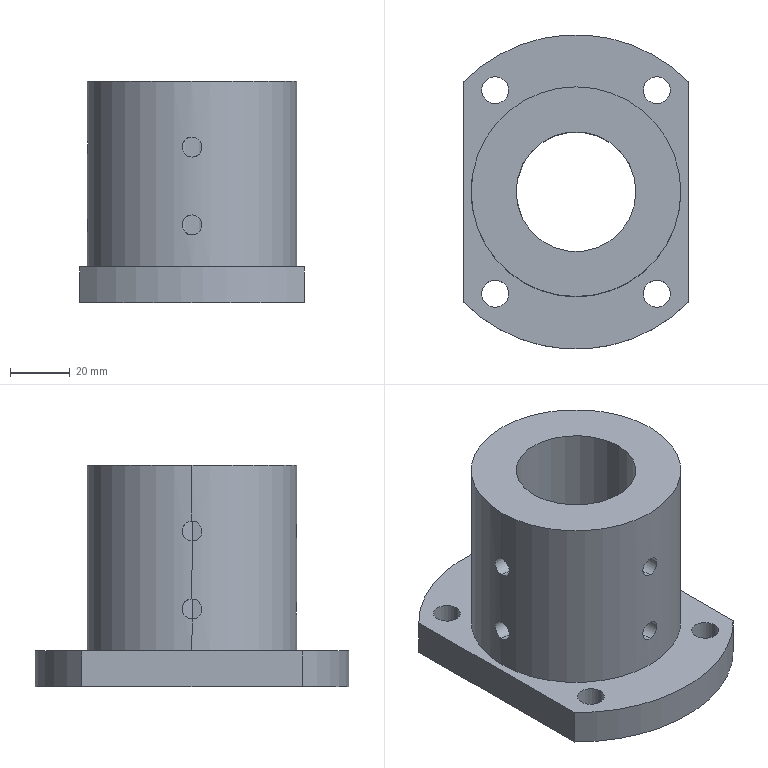Part | NX | features BREP 1 | 1 solid | 27 faces | box 75 x 105 x 74 mm | volume 226168 mm3 | cylinder 22 | plane 5 | commonest cylinder face diameters 6.647 x8 9 x8 40 x2 70 x2 105 x2
STEP:
#1=CARTESIAN_POINT('',(35.,0.,0.));
#2=VERTEX_POINT('',#1);
#3=CARTESIAN_POINT('',(-35.,0.,0.));
#4=VERTEX_POINT('',#3);
#5=CARTESIAN_POINT('',(0.,0.,0.));
#6=DIRECTION('',(0.,0.,1.));
#7=DIRECTION('',(1.,0.,0.));
#8=AXIS2_PLACEMENT_3D('',#5,#6,#7);
#9=CIRCLE('',#8,35.);
#10=EDGE_CURVE('',#2,#4,#9,.T.);
#11=ORIENTED_EDGE('',*,*,#10,.T.);
#12=CARTESIAN_POINT('',(-35.,0.,10.677));
#13=VERTEX_POINT('',#12);
#14=CARTESIAN_POINT('',(-35.,0.,0.));
#15=DIRECTION('',(0.,0.,1.));
#16=VECTOR('',#15,1000.);
#17=LINE('',#14,#16);
#18=EDGE_CURVE('',#4,#13,#17,.T.);
#19=ORIENTED_EDGE('',*,*,#18,.T.);
#20=CARTESIAN_POINT('',(-35.,0.,17.323));
#21=VERTEX_POINT('',#20);
#22=CARTESIAN_POINT('',(-35.,0.,10.677));
#23=CARTESIAN_POINT('',(-35.,0.874,10.677));
#24=CARTESIAN_POINT('',(-34.921,2.604,11.398));
#25=CARTESIAN_POINT('',(-34.802,3.684,14.));
#26=CARTESIAN_POINT('',(-34.921,2.603,16.603));
#27=CARTESIAN_POINT('',(-35.,0.8744,17.323));
#28=CARTESIAN_POINT('',(-35.,0.,17.323));
#29=B_SPLINE_CURVE_WITH_KNOTS('',3,(#22,#23,#24,#25,#26,#27,#28),.UNSPECIFIED.,.F.,.F.,(4,1,1,1,4),(0.,0.25,0.5,0.75,1.),.UNSPECIFIED.);
#30=EDGE_CURVE('',#13,#21,#29,.T.);
#31=ORIENTED_EDGE('',*,*,#30,.T.);
#32=CARTESIAN_POINT('',(-35.,0.,36.676));
#33=VERTEX_POINT('',#32);
#34=CARTESIAN_POINT('',(-35.,0.,0.));
#35=DIRECTION('',(0.,0.,1.));
#36=VECTOR('',#35,1000.);
#37=LINE('',#34,#36);
#38=EDGE_CURVE('',#21,#33,#37,.T.);
#39=ORIENTED_EDGE('',*,*,#38,.T.);
#40=CARTESIAN_POINT('',(-35.,0.,43.324));
#41=VERTEX_POINT('',#40);
#42=CARTESIAN_POINT('',(-35.,0.,36.676));
#43=CARTESIAN_POINT('',(-35.,0.874,36.676));
#44=CARTESIAN_POINT('',(-34.921,2.604,37.398));
#45=CARTESIAN_POINT('',(-34.802,3.684,40.));
#46=CARTESIAN_POINT('',(-34.921,2.603,42.603));
#47=CARTESIAN_POINT('',(-35.,0.8744,43.324));
#48=CARTESIAN_POINT('',(-35.,0.,43.324));
#49=B_SPLINE_CURVE_WITH_KNOTS('',3,(#42,#43,#44,#45,#46,#47,#48),.UNSPECIFIED.,.F.,.F.,(4,1,1,1,4),(0.,0.25,0.5,0.75,1.),.UNSPECIFIED.);
#50=EDGE_CURVE('',#33,#41,#49,.T.);
#51=ORIENTED_EDGE('',*,*,#50,.T.);
#52=CARTESIAN_POINT('',(-35.,0.,62.));
#53=VERTEX_POINT('',#52);
#54=CARTESIAN_POINT('',(-35.,0.,0.));
#55=DIRECTION('',(0.,0.,1.));
#56=VECTOR('',#55,1000.);
#57=LINE('',#54,#56);
#58=EDGE_CURVE('',#53,#41,#57,.F.);
#59=ORIENTED_EDGE('',*,*,#58,.F.);
#60=CARTESIAN_POINT('',(35.,0.,62.));
#61=VERTEX_POINT('',#60);
#62=CARTESIAN_POINT('',(0.,0.,62.));
#63=DIRECTION('',(0.,0.,-1.));
#64=DIRECTION('',(1.,0.,0.));
#65=AXIS2_PLACEMENT_3D('',#62,#63,#64);
#66=CIRCLE('',#65,35.);
#67=EDGE_CURVE('',#53,#61,#66,.T.);
#68=ORIENTED_EDGE('',*,*,#67,.T.);
#69=CARTESIAN_POINT('',(35.,0.,0.));
#70=DIRECTION('',(0.,0.,1.));
#71=VECTOR('',#70,1000.);
#72=LINE('',#69,#71);
#73=EDGE_CURVE('',#61,#2,#72,.F.);
#74=ORIENTED_EDGE('',*,*,#73,.T.);
#75=EDGE_LOOP('',(#11,#19,#31,#39,#51,#59,#68,#74));
#76=FACE_BOUND('',#75,.T.);
#77=CARTESIAN_POINT('',(0.,0.,0.));
#78=DIRECTION('',(0.,0.,1.));
#79=DIRECTION('',(1.,0.,0.));
#80=AXIS2_PLACEMENT_3D('',#77,#78,#79);
#81=CYLINDRICAL_SURFACE('',#80,35.);
#82=ADVANCED_FACE('',(#76),#81,.T.);
#83=CARTESIAN_POINT('',(-20.,0.,36.676));
#84=VERTEX_POINT('',#83);
#85=CARTESIAN_POINT('',(-20.,0.,43.324));
#86=VERTEX_POINT('',#85);
#87=CARTESIAN_POINT('',(-20.,0.,43.324));
#88=CARTESIAN_POINT('',(-20.,-0.2063,43.324));
#89=CARTESIAN_POINT('',(-19.994,-0.6164,43.293));
#90=CARTESIAN_POINT('',(-19.959,-1.329,43.064));
#91=CARTESIAN_POINT('',(-19.927,-1.717,42.865));
#92=CARTESIAN_POINT('',(-19.862,-2.379,42.381));
#93=CARTESIAN_POINT('',(-19.795,-2.871,41.708));
#94=CARTESIAN_POINT('',(-19.764,-3.064,41.328));
#95=CARTESIAN_POINT('',(-19.727,-3.294,40.612));
#96=CARTESIAN_POINT('',(-19.719,-3.338,39.997));
#97=CARTESIAN_POINT('',(-19.728,-3.294,39.383));
#98=CARTESIAN_POINT('',(-19.764,-3.063,38.669));
#99=CARTESIAN_POINT('',(-19.795,-2.87,38.29));
#100=CARTESIAN_POINT('',(-19.862,-2.377,37.617));
#101=CARTESIAN_POINT('',(-19.928,-1.716,37.134));
#102=CARTESIAN_POINT('',(-19.959,-1.326,36.935));
#103=CARTESIAN_POINT('',(-19.994,-0.6156,36.707));
#104=CARTESIAN_POINT('',(-20.,-0.206,36.676));
#105=CARTESIAN_POINT('',(-20.,0.,36.676));
#106=B_SPLINE_CURVE_WITH_KNOTS('',3,(#87,#88,#89,#90,#91,#92,#93,#94,#95,#96,#97,#98,#99,#100,#101,#102,#103,#104,#105),.UNSPECIFIED.,.F.,.F.,(4,1,1,1,1,1,1,1,1,1,1,1,1,1,1,1,4),(0.,0.0625,0.125,0.1875,0.25,0.3125,0.375,0.4375,0.5,0.5625,0.625,0.6875,0.75,0.8125,0.875,0.9375,1.),.UNSPECIFIED.);
#107=EDGE_CURVE('',#84,#86,#106,.F.);
#108=ORIENTED_EDGE('',*,*,#107,.F.);
#109=CARTESIAN_POINT('',(0.,0.,36.676));
#110=DIRECTION('',(-1.,0.,0.));
#111=VECTOR('',#110,1000.);
#112=LINE('',#109,#111);
#113=EDGE_CURVE('',#33,#84,#112,.F.);
#114=ORIENTED_EDGE('',*,*,#113,.F.);
#115=CARTESIAN_POINT('',(-35.,0.,36.676));
#116=CARTESIAN_POINT('',(-35.,-0.206,36.676));
#117=CARTESIAN_POINT('',(-34.997,-0.6155,36.706));
#118=CARTESIAN_POINT('',(-34.976,-1.328,36.936));
#119=CARTESIAN_POINT('',(-34.959,-1.714,37.133));
#120=CARTESIAN_POINT('',(-34.921,-2.38,37.62));
#121=CARTESIAN_POINT('',(-34.883,-2.87,38.29));
#122=CARTESIAN_POINT('',(-34.865,-3.066,38.675));
#123=CARTESIAN_POINT('',(-34.845,-3.294,39.388));
#124=CARTESIAN_POINT('',(-34.84,-3.338,40.003));
#125=CARTESIAN_POINT('',(-34.845,-3.293,40.617));
#126=CARTESIAN_POINT('',(-34.866,-3.064,41.329));
#127=CARTESIAN_POINT('',(-34.883,-2.868,41.712));
#128=CARTESIAN_POINT('',(-34.921,-2.378,42.382));
#129=CARTESIAN_POINT('',(-34.959,-1.713,42.868));
#130=CARTESIAN_POINT('',(-34.976,-1.326,43.065));
#131=CARTESIAN_POINT('',(-34.997,-0.6147,43.294));
#132=CARTESIAN_POINT('',(-35.,-0.2057,43.324));
#133=CARTESIAN_POINT('',(-35.,0.,43.324));
#134=B_SPLINE_CURVE_WITH_KNOTS('',3,(#115,#116,#117,#118,#119,#120,#121,#122,#123,#124,#125,#126,#127,#128,#129,#130,#131,#132,#133),.UNSPECIFIED.,.F.,.F.,(4,1,1,1,1,1,1,1,1,1,1,1,1,1,1,1,4),(0.,0.0625,0.125,0.1875,0.25,0.3125,0.375,0.4375,0.5,0.5625,0.625,0.6875,0.75,0.8125,0.875,0.9375,1.),.UNSPECIFIED.);
#135=EDGE_CURVE('',#41,#33,#134,.F.);
#136=ORIENTED_EDGE('',*,*,#135,.F.);
#137=CARTESIAN_POINT('',(0.,0.,43.324));
#138=DIRECTION('',(-1.,0.,0.));
#139=VECTOR('',#138,1000.);
#140=LINE('',#137,#139);
#141=EDGE_CURVE('',#41,#86,#140,.F.);
#142=ORIENTED_EDGE('',*,*,#141,.T.);
#143=EDGE_LOOP('',(#108,#114,#136,#142));
#144=FACE_BOUND('',#143,.T.);
#145=CARTESIAN_POINT('',(0.,0.,40.));
#146=DIRECTION('',(-1.,0.,0.));
#147=DIRECTION('',(0.,0.,1.));
#148=AXIS2_PLACEMENT_3D('',#145,#146,#147);
#149=CYLINDRICAL_SURFACE('',#148,3.324);
#150=ADVANCED_FACE('',(#144),#149,.F.);
#151=CARTESIAN_POINT('',(0.,-20.,17.323));
#152=VERTEX_POINT('',#151);
#153=CARTESIAN_POINT('',(0.,-20.,10.676));
#154=VERTEX_POINT('',#153);
#155=CARTESIAN_POINT('',(0.,-20.,10.677));
#156=CARTESIAN_POINT('',(-0.4121,-20.,10.677));
#157=CARTESIAN_POINT('',(-1.02,-19.978,10.806));
#158=CARTESIAN_POINT('',(-1.541,-19.941,11.048));
#159=CARTESIAN_POINT('',(-1.874,-19.913,11.249));
#160=CARTESIAN_POINT('',(-2.049,-19.895,11.379));
#161=CARTESIAN_POINT('',(-2.357,-19.862,11.641));
#162=CARTESIAN_POINT('',(-2.63,-19.827,11.961));
#163=CARTESIAN_POINT('',(-2.748,-19.81,12.123));
#164=CARTESIAN_POINT('',(-2.952,-19.781,12.46));
#165=CARTESIAN_POINT('',(-3.111,-19.757,12.804));
#166=CARTESIAN_POINT('',(-3.291,-19.728,13.382));
#167=CARTESIAN_POINT('',(-3.34,-19.719,14.));
#168=CARTESIAN_POINT('',(-3.291,-19.728,14.618));
#169=CARTESIAN_POINT('',(-3.111,-19.757,15.196));
#170=CARTESIAN_POINT('',(-2.953,-19.781,15.54));
#171=CARTESIAN_POINT('',(-2.748,-19.81,15.877));
#172=CARTESIAN_POINT('',(-2.629,-19.827,16.039));
#173=CARTESIAN_POINT('',(-2.358,-19.861,16.357));
#174=CARTESIAN_POINT('',(-2.046,-19.895,16.624));
#175=CARTESIAN_POINT('',(-1.874,-19.913,16.75));
#176=CARTESIAN_POINT('',(-1.543,-19.941,16.951));
#177=CARTESIAN_POINT('',(-1.019,-19.978,17.194));
#178=CARTESIAN_POINT('',(-0.4124,-20.,17.323));
#179=CARTESIAN_POINT('',(0.,-20.,17.323));
#180=B_SPLINE_CURVE_WITH_KNOTS('',3,(#155,#156,#157,#158,#159,#160,#161,#162,#163,#164,#165,#166,#167,#168,#169,#170,#171,#172,#173,#174,#175,#176,#177,#178,#179),.UNSPECIFIED.,.F.,.F.,(4,1,1,1,1,1,1,1,1,1,1,1,1,1,1,1,1,1,1,1,1,1,4),(0.,0.125,0.1562,0.1875,0.2188,0.25,0.2812,0.3125,0.3438,0.375,0.4375,0.5,0.5625,0.625,0.6562,0.6875,0.7188,0.75,0.7812,0.8125,0.8438,0.875,1.),.UNSPECIFIED.);
#181=EDGE_CURVE('',#152,#154,#180,.F.);
#182=ORIENTED_EDGE('',*,*,#181,.F.);
#183=CARTESIAN_POINT('',(0.,-35.,17.323));
#184=VERTEX_POINT('',#183);
#185=CARTESIAN_POINT('',(0.,0.,17.323));
#186=DIRECTION('',(0.,-1.,0.));
#187=VECTOR('',#186,1000.);
#188=LINE('',#185,#187);
#189=EDGE_CURVE('',#152,#184,#188,.T.);
#190=ORIENTED_EDGE('',*,*,#189,.T.);
#191=CARTESIAN_POINT('',(0.,-35.,10.677));
#192=VERTEX_POINT('',#191);
#193=CARTESIAN_POINT('',(0.,-35.,17.323));
#194=CARTESIAN_POINT('',(-0.206,-35.,17.323));
#195=CARTESIAN_POINT('',(-0.6155,-34.997,17.294));
#196=CARTESIAN_POINT('',(-1.328,-34.976,17.064));
#197=CARTESIAN_POINT('',(-1.714,-34.959,16.867));
#198=CARTESIAN_POINT('',(-2.38,-34.921,16.38));
#199=CARTESIAN_POINT('',(-2.87,-34.883,15.71));
#200=CARTESIAN_POINT('',(-3.066,-34.865,15.325));
#201=CARTESIAN_POINT('',(-3.294,-34.845,14.612));
#202=CARTESIAN_POINT('',(-3.338,-34.84,13.997));
#203=CARTESIAN_POINT('',(-3.293,-34.845,13.383));
#204=CARTESIAN_POINT('',(-3.064,-34.866,12.671));
#205=CARTESIAN_POINT('',(-2.868,-34.883,12.288));
#206=CARTESIAN_POINT('',(-2.378,-34.921,11.618));
#207=CARTESIAN_POINT('',(-1.713,-34.959,11.132));
#208=CARTESIAN_POINT('',(-1.326,-34.976,10.935));
#209=CARTESIAN_POINT('',(-0.6147,-34.997,10.706));
#210=CARTESIAN_POINT('',(-0.2057,-35.,10.677));
#211=CARTESIAN_POINT('',(0.,-35.,10.677));
#212=B_SPLINE_CURVE_WITH_KNOTS('',3,(#193,#194,#195,#196,#197,#198,#199,#200,#201,#202,#203,#204,#205,#206,#207,#208,#209,#210,#211),.UNSPECIFIED.,.F.,.F.,(4,1,1,1,1,1,1,1,1,1,1,1,1,1,1,1,4),(0.,0.0625,0.125,0.1875,0.25,0.3125,0.375,0.4375,0.5,0.5625,0.625,0.6875,0.75,0.8125,0.875,0.9375,1.),.UNSPECIFIED.);
#213=EDGE_CURVE('',#192,#184,#212,.F.);
#214=ORIENTED_EDGE('',*,*,#213,.F.);
#215=CARTESIAN_POINT('',(0.,0.,10.677));
#216=DIRECTION('',(0.,-1.,0.));
#217=VECTOR('',#216,1000.);
#218=LINE('',#215,#217);
#219=EDGE_CURVE('',#154,#192,#218,.T.);
#220=ORIENTED_EDGE('',*,*,#219,.F.);
#221=EDGE_LOOP('',(#182,#190,#214,#220));
#222=FACE_BOUND('',#221,.T.);
#223=CARTESIAN_POINT('',(0.,0.,14.));
#224=DIRECTION('',(0.,-1.,0.));
#225=DIRECTION('',(0.,0.,-1.));
#226=AXIS2_PLACEMENT_3D('',#223,#224,#225);
#227=CYLINDRICAL_SURFACE('',#226,3.324);
#228=ADVANCED_FACE('',(#222),#227,.F.);
#229=CARTESIAN_POINT('',(-20.,0.,10.676));
#230=VERTEX_POINT('',#229);
#231=CARTESIAN_POINT('',(-20.,0.,17.323));
#232=VERTEX_POINT('',#231);
#233=CARTESIAN_POINT('',(-20.,0.,17.323));
#234=CARTESIAN_POINT('',(-20.,-0.2063,17.323));
#235=CARTESIAN_POINT('',(-19.994,-0.6164,17.293));
#236=CARTESIAN_POINT('',(-19.959,-1.329,17.064));
#237=CARTESIAN_POINT('',(-19.927,-1.717,16.865));
#238=CARTESIAN_POINT('',(-19.862,-2.379,16.381));
#239=CARTESIAN_POINT('',(-19.795,-2.871,15.708));
#240=CARTESIAN_POINT('',(-19.764,-3.064,15.328));
#241=CARTESIAN_POINT('',(-19.727,-3.294,14.612));
#242=CARTESIAN_POINT('',(-19.719,-3.338,13.997));
#243=CARTESIAN_POINT('',(-19.728,-3.294,13.383));
#244=CARTESIAN_POINT('',(-19.764,-3.063,12.669));
#245=CARTESIAN_POINT('',(-19.795,-2.87,12.29));
#246=CARTESIAN_POINT('',(-19.862,-2.377,11.617));
#247=CARTESIAN_POINT('',(-19.928,-1.716,11.134));
#248=CARTESIAN_POINT('',(-19.959,-1.326,10.935));
#249=CARTESIAN_POINT('',(-19.994,-0.6156,10.707));
#250=CARTESIAN_POINT('',(-20.,-0.206,10.677));
#251=CARTESIAN_POINT('',(-20.,0.,10.677));
#252=B_SPLINE_CURVE_WITH_KNOTS('',3,(#233,#234,#235,#236,#237,#238,#239,#240,#241,#242,#243,#244,#245,#246,#247,#248,#249,#250,#251),.UNSPECIFIED.,.F.,.F.,(4,1,1,1,1,1,1,1,1,1,1,1,1,1,1,1,4),(0.,0.0625,0.125,0.1875,0.25,0.3125,0.375,0.4375,0.5,0.5625,0.625,0.6875,0.75,0.8125,0.875,0.9375,1.),.UNSPECIFIED.);
#253=EDGE_CURVE('',#230,#232,#252,.F.);
#254=ORIENTED_EDGE('',*,*,#253,.F.);
#255=CARTESIAN_POINT('',(0.,0.,10.677));
#256=DIRECTION('',(-1.,0.,0.));
#257=VECTOR('',#256,1000.);
#258=LINE('',#255,#257);
#259=EDGE_CURVE('',#13,#230,#258,.F.);
#260=ORIENTED_EDGE('',*,*,#259,.F.);
#261=CARTESIAN_POINT('',(-35.,0.,10.677));
#262=CARTESIAN_POINT('',(-35.,-0.206,10.677));
#263=CARTESIAN_POINT('',(-34.997,-0.6155,10.706));
#264=CARTESIAN_POINT('',(-34.976,-1.328,10.936));
#265=CARTESIAN_POINT('',(-34.959,-1.714,11.133));
#266=CARTESIAN_POINT('',(-34.921,-2.38,11.62));
#267=CARTESIAN_POINT('',(-34.883,-2.87,12.29));
#268=CARTESIAN_POINT('',(-34.865,-3.066,12.675));
#269=CARTESIAN_POINT('',(-34.845,-3.294,13.388));
#270=CARTESIAN_POINT('',(-34.84,-3.338,14.003));
#271=CARTESIAN_POINT('',(-34.845,-3.293,14.617));
#272=CARTESIAN_POINT('',(-34.866,-3.064,15.329));
#273=CARTESIAN_POINT('',(-34.883,-2.868,15.712));
#274=CARTESIAN_POINT('',(-34.921,-2.378,16.382));
#275=CARTESIAN_POINT('',(-34.959,-1.713,16.868));
#276=CARTESIAN_POINT('',(-34.976,-1.326,17.065));
#277=CARTESIAN_POINT('',(-34.997,-0.6147,17.294));
#278=CARTESIAN_POINT('',(-35.,-0.2057,17.323));
#279=CARTESIAN_POINT('',(-35.,0.,17.323));
#280=B_SPLINE_CURVE_WITH_KNOTS('',3,(#261,#262,#263,#264,#265,#266,#267,#268,#269,#270,#271,#272,#273,#274,#275,#276,#277,#278,#279),.UNSPECIFIED.,.F.,.F.,(4,1,1,1,1,1,1,1,1,1,1,1,1,1,1,1,4),(0.,0.0625,0.125,0.1875,0.25,0.3125,0.375,0.4375,0.5,0.5625,0.625,0.6875,0.75,0.8125,0.875,0.9375,1.),.UNSPECIFIED.);
#281=EDGE_CURVE('',#21,#13,#280,.F.);
#282=ORIENTED_EDGE('',*,*,#281,.F.);
#283=CARTESIAN_POINT('',(0.,0.,17.323));
#284=DIRECTION('',(-1.,0.,0.));
#285=VECTOR('',#284,1000.);
#286=LINE('',#283,#285);
#287=EDGE_CURVE('',#21,#232,#286,.F.);
#288=ORIENTED_EDGE('',*,*,#287,.T.);
#289=EDGE_LOOP('',(#254,#260,#282,#288));
#290=FACE_BOUND('',#289,.T.);
#291=CARTESIAN_POINT('',(0.,0.,14.));
#292=DIRECTION('',(-1.,0.,0.));
#293=DIRECTION('',(0.,0.,1.));
#294=AXIS2_PLACEMENT_3D('',#291,#292,#293);
#295=CYLINDRICAL_SURFACE('',#294,3.324);
#296=ADVANCED_FACE('',(#290),#295,.F.);
#297=CARTESIAN_POINT('',(0.,-20.,43.324));
#298=VERTEX_POINT('',#297);
#299=CARTESIAN_POINT('',(0.,-20.,36.676));
#300=VERTEX_POINT('',#299);
#301=CARTESIAN_POINT('',(0.,-20.,36.676));
#302=CARTESIAN_POINT('',(-0.4121,-20.,36.676));
#303=CARTESIAN_POINT('',(-1.02,-19.978,36.806));
#304=CARTESIAN_POINT('',(-1.541,-19.941,37.048));
#305=CARTESIAN_POINT('',(-1.874,-19.913,37.249));
#306=CARTESIAN_POINT('',(-2.049,-19.895,37.379));
#307=CARTESIAN_POINT('',(-2.357,-19.862,37.641));
#308=CARTESIAN_POINT('',(-2.63,-19.827,37.961));
#309=CARTESIAN_POINT('',(-2.748,-19.81,38.123));
#310=CARTESIAN_POINT('',(-2.952,-19.781,38.46));
#311=CARTESIAN_POINT('',(-3.111,-19.757,38.804));
#312=CARTESIAN_POINT('',(-3.291,-19.728,39.382));
#313=CARTESIAN_POINT('',(-3.34,-19.719,40.));
#314=CARTESIAN_POINT('',(-3.291,-19.728,40.618));
#315=CARTESIAN_POINT('',(-3.111,-19.757,41.196));
#316=CARTESIAN_POINT('',(-2.953,-19.781,41.54));
#317=CARTESIAN_POINT('',(-2.748,-19.81,41.877));
#318=CARTESIAN_POINT('',(-2.629,-19.827,42.039));
#319=CARTESIAN_POINT('',(-2.358,-19.861,42.357));
#320=CARTESIAN_POINT('',(-2.046,-19.895,42.624));
#321=CARTESIAN_POINT('',(-1.874,-19.913,42.75));
#322=CARTESIAN_POINT('',(-1.543,-19.941,42.951));
#323=CARTESIAN_POINT('',(-1.019,-19.978,43.194));
#324=CARTESIAN_POINT('',(-0.4124,-20.,43.324));
#325=CARTESIAN_POINT('',(0.,-20.,43.324));
#326=B_SPLINE_CURVE_WITH_KNOTS('',3,(#301,#302,#303,#304,#305,#306,#307,#308,#309,#310,#311,#312,#313,#314,#315,#316,#317,#318,#319,#320,#321,#322,#323,#324,#325),.UNSPECIFIED.,.F.,.F.,(4,1,1,1,1,1,1,1,1,1,1,1,1,1,1,1,1,1,1,1,1,1,4),(0.,0.125,0.1562,0.1875,0.2188,0.25,0.2812,0.3125,0.3438,0.375,0.4375,0.5,0.5625,0.625,0.6562,0.6875,0.7188,0.75,0.7812,0.8125,0.8438,0.875,1.),.UNSPECIFIED.);
#327=EDGE_CURVE('',#298,#300,#326,.F.);
#328=ORIENTED_EDGE('',*,*,#327,.F.);
#329=CARTESIAN_POINT('',(0.,-35.,43.324));
#330=VERTEX_POINT('',#329);
#331=CARTESIAN_POINT('',(0.,0.,43.324));
#332=DIRECTION('',(0.,-1.,0.));
#333=VECTOR('',#332,1000.);
#334=LINE('',#331,#333);
#335=EDGE_CURVE('',#298,#330,#334,.T.);
#336=ORIENTED_EDGE('',*,*,#335,.T.);
#337=CARTESIAN_POINT('',(0.,-35.,36.676));
#338=VERTEX_POINT('',#337);
#339=CARTESIAN_POINT('',(0.,-35.,43.324));
#340=CARTESIAN_POINT('',(-0.206,-35.,43.324));
#341=CARTESIAN_POINT('',(-0.6155,-34.997,43.294));
#342=CARTESIAN_POINT('',(-1.328,-34.976,43.064));
#343=CARTESIAN_POINT('',(-1.714,-34.959,42.867));
#344=CARTESIAN_POINT('',(-2.38,-34.921,42.38));
#345=CARTESIAN_POINT('',(-2.87,-34.883,41.71));
#346=CARTESIAN_POINT('',(-3.066,-34.865,41.325));
#347=CARTESIAN_POINT('',(-3.294,-34.845,40.612));
#348=CARTESIAN_POINT('',(-3.338,-34.84,39.997));
#349=CARTESIAN_POINT('',(-3.293,-34.845,39.383));
#350=CARTESIAN_POINT('',(-3.064,-34.866,38.671));
#351=CARTESIAN_POINT('',(-2.868,-34.883,38.288));
#352=CARTESIAN_POINT('',(-2.378,-34.921,37.618));
#353=CARTESIAN_POINT('',(-1.713,-34.959,37.132));
#354=CARTESIAN_POINT('',(-1.326,-34.976,36.935));
#355=CARTESIAN_POINT('',(-0.6147,-34.997,36.706));
#356=CARTESIAN_POINT('',(-0.2057,-35.,36.676));
#357=CARTESIAN_POINT('',(0.,-35.,36.676));
#358=B_SPLINE_CURVE_WITH_KNOTS('',3,(#339,#340,#341,#342,#343,#344,#345,#346,#347,#348,#349,#350,#351,#352,#353,#354,#355,#356,#357),.UNSPECIFIED.,.F.,.F.,(4,1,1,1,1,1,1,1,1,1,1,1,1,1,1,1,4),(0.,0.0625,0.125,0.1875,0.25,0.3125,0.375,0.4375,0.5,0.5625,0.625,0.6875,0.75,0.8125,0.875,0.9375,1.),.UNSPECIFIED.);
#359=EDGE_CURVE('',#338,#330,#358,.F.);
#360=ORIENTED_EDGE('',*,*,#359,.F.);
#361=CARTESIAN_POINT('',(0.,0.,36.676));
#362=DIRECTION('',(0.,-1.,0.));
#363=VECTOR('',#362,1000.);
#364=LINE('',#361,#363);
#365=EDGE_CURVE('',#300,#338,#364,.T.);
#366=ORIENTED_EDGE('',*,*,#365,.F.);
#367=EDGE_LOOP('',(#328,#336,#360,#366));
#368=FACE_BOUND('',#367,.T.);
#369=CARTESIAN_POINT('',(0.,0.,40.));
#370=DIRECTION('',(0.,-1.,0.));
#371=DIRECTION('',(0.,0.,-1.));
#372=AXIS2_PLACEMENT_3D('',#369,#370,#371);
#373=CYLINDRICAL_SURFACE('',#372,3.324);
#374=ADVANCED_FACE('',(#368),#373,.F.);
#375=CARTESIAN_POINT('',(-20.,0.,-12.));
#376=VERTEX_POINT('',#375);
#377=CARTESIAN_POINT('',(20.,0.,-12.));
#378=VERTEX_POINT('',#377);
#379=CARTESIAN_POINT('',(0.,0.,-12.));
#380=DIRECTION('',(0.,0.,1.));
#381=DIRECTION('',(1.,0.,0.));
#382=AXIS2_PLACEMENT_3D('',#379,#380,#381);
#383=CIRCLE('',#382,20.);
#384=EDGE_CURVE('',#376,#378,#383,.T.);
#385=ORIENTED_EDGE('',*,*,#384,.F.);
#386=CARTESIAN_POINT('',(-20.,0.,0.));
#387=DIRECTION('',(0.,0.,1.));
#388=VECTOR('',#387,1000.);
#389=LINE('',#386,#388);
#390=EDGE_CURVE('',#376,#230,#389,.T.);
#391=ORIENTED_EDGE('',*,*,#390,.T.);
#392=ORIENTED_EDGE('',*,*,#253,.T.);
#393=CARTESIAN_POINT('',(-20.,0.,0.));
#394=DIRECTION('',(0.,0.,1.));
#395=VECTOR('',#394,1000.);
#396=LINE('',#393,#395);
#397=EDGE_CURVE('',#232,#84,#396,.T.);
#398=ORIENTED_EDGE('',*,*,#397,.T.);
#399=ORIENTED_EDGE('',*,*,#107,.T.);
#400=CARTESIAN_POINT('',(-20.,0.,62.));
#401=VERTEX_POINT('',#400);
#402=CARTESIAN_POINT('',(-20.,0.,0.));
#403=DIRECTION('',(0.,0.,1.));
#404=VECTOR('',#403,1000.);
#405=LINE('',#402,#404);
#406=EDGE_CURVE('',#401,#86,#405,.F.);
#407=ORIENTED_EDGE('',*,*,#406,.F.);
#408=CARTESIAN_POINT('',(20.,0.,62.));
#409=VERTEX_POINT('',#408);
#410=CARTESIAN_POINT('',(0.,0.,62.));
#411=DIRECTION('',(0.,0.,-1.));
#412=DIRECTION('',(1.,0.,0.));
#413=AXIS2_PLACEMENT_3D('',#410,#411,#412);
#414=CIRCLE('',#413,20.);
#415=EDGE_CURVE('',#409,#401,#414,.T.);
#416=ORIENTED_EDGE('',*,*,#415,.F.);
#417=CARTESIAN_POINT('',(20.,0.,0.));
#418=DIRECTION('',(0.,0.,1.));
#419=VECTOR('',#418,1000.);
#420=LINE('',#417,#419);
#421=EDGE_CURVE('',#409,#378,#420,.F.);
#422=ORIENTED_EDGE('',*,*,#421,.T.);
#423=EDGE_LOOP('',(#385,#391,#392,#398,#399,#407,#416,#422));
#424=FACE_BOUND('',#423,.T.);
#425=CARTESIAN_POINT('',(0.,-20.,36.676));
#426=CARTESIAN_POINT('',(0.8815,-20.,36.676));
#427=CARTESIAN_POINT('',(2.596,-19.862,37.395));
#428=CARTESIAN_POINT('',(3.687,-19.652,39.996));
#429=CARTESIAN_POINT('',(2.598,-19.862,42.604));
#430=CARTESIAN_POINT('',(0.8833,-20.,43.324));
#431=CARTESIAN_POINT('',(0.,-20.,43.324));
#432=B_SPLINE_CURVE_WITH_KNOTS('',3,(#425,#426,#427,#428,#429,#430,#431),.UNSPECIFIED.,.F.,.F.,(4,1,1,1,4),(0.,0.25,0.5,0.75,1.),.UNSPECIFIED.);
#433=EDGE_CURVE('',#300,#298,#432,.T.);
#434=ORIENTED_EDGE('',*,*,#433,.T.);
#435=ORIENTED_EDGE('',*,*,#327,.T.);
#436=EDGE_LOOP('',(#434,#435));
#437=FACE_BOUND('',#436,.T.);
#438=CARTESIAN_POINT('',(0.,-20.,10.676));
#439=CARTESIAN_POINT('',(0.8815,-20.,10.676));
#440=CARTESIAN_POINT('',(2.596,-19.862,11.395));
#441=CARTESIAN_POINT('',(3.687,-19.652,13.996));
#442=CARTESIAN_POINT('',(2.598,-19.862,16.604));
#443=CARTESIAN_POINT('',(0.8833,-20.,17.323));
#444=CARTESIAN_POINT('',(0.,-20.,17.323));
#445=B_SPLINE_CURVE_WITH_KNOTS('',3,(#438,#439,#440,#441,#442,#443,#444),.UNSPECIFIED.,.F.,.F.,(4,1,1,1,4),(0.,0.25,0.5,0.75,1.),.UNSPECIFIED.);
#446=EDGE_CURVE('',#154,#152,#445,.T.);
#447=ORIENTED_EDGE('',*,*,#446,.T.);
#448=ORIENTED_EDGE('',*,*,#181,.T.);
#449=EDGE_LOOP('',(#447,#448));
#450=FACE_BOUND('',#449,.T.);
#451=CARTESIAN_POINT('',(0.,0.,0.));
#452=DIRECTION('',(0.,0.,1.));
#453=DIRECTION('',(1.,0.,0.));
#454=AXIS2_PLACEMENT_3D('',#451,#452,#453);
#455=CYLINDRICAL_SURFACE('',#454,20.);
#456=ADVANCED_FACE('',(#424,#437,#450),#455,.F.);
#457=CARTESIAN_POINT('',(31.5,34.,0.));
#458=VERTEX_POINT('',#457);
#459=CARTESIAN_POINT('',(22.5,34.,0.));
#460=VERTEX_POINT('',#459);
#461=CARTESIAN_POINT('',(27.,34.,0.));
#462=DIRECTION('',(0.,0.,-1.));
#463=DIRECTION('',(-1.,0.,0.));
#464=AXIS2_PLACEMENT_3D('',#461,#462,#463);
#465=CIRCLE('',#464,4.5);
#466=EDGE_CURVE('',#458,#460,#465,.T.);
#467=ORIENTED_EDGE('',*,*,#466,.F.);
#468=CARTESIAN_POINT('',(31.5,34.,-12.));
#469=VERTEX_POINT('',#468);
#470=CARTESIAN_POINT('',(31.5,34.,-12.));
#471=DIRECTION('',(0.,0.,-1.));
#472=VECTOR('',#471,1000.);
#473=LINE('',#470,#472);
#474=EDGE_CURVE('',#458,#469,#473,.T.);
#475=ORIENTED_EDGE('',*,*,#474,.T.);
#476=CARTESIAN_POINT('',(22.5,34.,-12.));
#477=VERTEX_POINT('',#476);
#478=CARTESIAN_POINT('',(27.,34.,-12.));
#479=DIRECTION('',(0.,0.,1.));
#480=DIRECTION('',(-1.,0.,0.));
#481=AXIS2_PLACEMENT_3D('',#478,#479,#480);
#482=CIRCLE('',#481,4.5);
#483=EDGE_CURVE('',#477,#469,#482,.T.);
#484=ORIENTED_EDGE('',*,*,#483,.F.);
#485=CARTESIAN_POINT('',(22.5,34.,-12.));
#486=DIRECTION('',(0.,0.,-1.));
#487=VECTOR('',#486,1000.);
#488=LINE('',#485,#487);
#489=EDGE_CURVE('',#460,#477,#488,.T.);
#490=ORIENTED_EDGE('',*,*,#489,.F.);
#491=EDGE_LOOP('',(#467,#475,#484,#490));
#492=FACE_BOUND('',#491,.T.);
#493=CARTESIAN_POINT('',(27.,34.,-12.));
#494=DIRECTION('',(0.,0.,-1.));
#495=DIRECTION('',(-1.,0.,0.));
#496=AXIS2_PLACEMENT_3D('',#493,#494,#495);
#497=CYLINDRICAL_SURFACE('',#496,4.5);
#498=ADVANCED_FACE('',(#492),#497,.F.);
#499=CARTESIAN_POINT('',(31.5,-34.,0.));
#500=VERTEX_POINT('',#499);
#501=CARTESIAN_POINT('',(22.5,-34.,0.));
#502=VERTEX_POINT('',#501);
#503=CARTESIAN_POINT('',(27.,-34.,0.));
#504=DIRECTION('',(0.,0.,-1.));
#505=DIRECTION('',(-1.,0.,0.));
#506=AXIS2_PLACEMENT_3D('',#503,#504,#505);
#507=CIRCLE('',#506,4.5);
#508=EDGE_CURVE('',#500,#502,#507,.T.);
#509=ORIENTED_EDGE('',*,*,#508,.F.);
#510=CARTESIAN_POINT('',(31.5,-34.,-12.));
#511=VERTEX_POINT('',#510);
#512=CARTESIAN_POINT('',(31.5,-34.,-12.));
#513=DIRECTION('',(0.,0.,-1.));
#514=VECTOR('',#513,1000.);
#515=LINE('',#512,#514);
#516=EDGE_CURVE('',#500,#511,#515,.T.);
#517=ORIENTED_EDGE('',*,*,#516,.T.);
#518=CARTESIAN_POINT('',(22.5,-34.,-12.));
#519=VERTEX_POINT('',#518);
#520=CARTESIAN_POINT('',(27.,-34.,-12.));
#521=DIRECTION('',(0.,0.,1.));
#522=DIRECTION('',(-1.,0.,0.));
#523=AXIS2_PLACEMENT_3D('',#520,#521,#522);
#524=CIRCLE('',#523,4.5);
#525=EDGE_CURVE('',#519,#511,#524,.T.);
#526=ORIENTED_EDGE('',*,*,#525,.F.);
#527=CARTESIAN_POINT('',(22.5,-34.,-12.));
#528=DIRECTION('',(0.,0.,-1.));
#529=VECTOR('',#528,1000.);
#530=LINE('',#527,#529);
#531=EDGE_CURVE('',#502,#519,#530,.T.);
#532=ORIENTED_EDGE('',*,*,#531,.F.);
#533=EDGE_LOOP('',(#509,#517,#526,#532));
#534=FACE_BOUND('',#533,.T.);
#535=CARTESIAN_POINT('',(27.,-34.,-12.));
#536=DIRECTION('',(0.,0.,-1.));
#537=DIRECTION('',(-1.,0.,0.));
#538=AXIS2_PLACEMENT_3D('',#535,#536,#537);
#539=CYLINDRICAL_SURFACE('',#538,4.5);
#540=ADVANCED_FACE('',(#534),#539,.F.);
#541=CARTESIAN_POINT('',(-22.5,-34.,0.));
#542=VERTEX_POINT('',#541);
#543=CARTESIAN_POINT('',(-31.5,-34.,0.));
#544=VERTEX_POINT('',#543);
#545=CARTESIAN_POINT('',(-27.,-34.,0.));
#546=DIRECTION('',(0.,0.,-1.));
#547=DIRECTION('',(-1.,0.,0.));
#548=AXIS2_PLACEMENT_3D('',#545,#546,#547);
#549=CIRCLE('',#548,4.5);
#550=EDGE_CURVE('',#542,#544,#549,.T.);
#551=ORIENTED_EDGE('',*,*,#550,.F.);
#552=CARTESIAN_POINT('',(-22.5,-34.,-12.));
#553=VERTEX_POINT('',#552);
#554=CARTESIAN_POINT('',(-22.5,-34.,-12.));
#555=DIRECTION('',(0.,0.,-1.));
#556=VECTOR('',#555,1000.);
#557=LINE('',#554,#556);
#558=EDGE_CURVE('',#542,#553,#557,.T.);
#559=ORIENTED_EDGE('',*,*,#558,.T.);
#560=CARTESIAN_POINT('',(-31.5,-34.,-12.));
#561=VERTEX_POINT('',#560);
#562=CARTESIAN_POINT('',(-27.,-34.,-12.));
#563=DIRECTION('',(0.,0.,1.));
#564=DIRECTION('',(-1.,0.,0.));
#565=AXIS2_PLACEMENT_3D('',#562,#563,#564);
#566=CIRCLE('',#565,4.5);
#567=EDGE_CURVE('',#561,#553,#566,.T.);
#568=ORIENTED_EDGE('',*,*,#567,.F.);
#569=CARTESIAN_POINT('',(-31.5,-34.,-12.));
#570=DIRECTION('',(0.,0.,-1.));
#571=VECTOR('',#570,1000.);
#572=LINE('',#569,#571);
#573=EDGE_CURVE('',#544,#561,#572,.T.);
#574=ORIENTED_EDGE('',*,*,#573,.F.);
#575=EDGE_LOOP('',(#551,#559,#568,#574));
#576=FACE_BOUND('',#575,.T.);
#577=CARTESIAN_POINT('',(-27.,-34.,-12.));
#578=DIRECTION('',(0.,0.,-1.));
#579=DIRECTION('',(-1.,0.,0.));
#580=AXIS2_PLACEMENT_3D('',#577,#578,#579);
#581=CYLINDRICAL_SURFACE('',#580,4.5);
#582=ADVANCED_FACE('',(#576),#581,.F.);
#583=CARTESIAN_POINT('',(-22.5,34.,0.));
#584=VERTEX_POINT('',#583);
#585=CARTESIAN_POINT('',(-31.5,34.,0.));
#586=VERTEX_POINT('',#585);
#587=CARTESIAN_POINT('',(-27.,34.,0.));
#588=DIRECTION('',(0.,0.,-1.));
#589=DIRECTION('',(-1.,0.,0.));
#590=AXIS2_PLACEMENT_3D('',#587,#588,#589);
#591=CIRCLE('',#590,4.5);
#592=EDGE_CURVE('',#584,#586,#591,.T.);
#593=ORIENTED_EDGE('',*,*,#592,.F.);
#594=CARTESIAN_POINT('',(-22.5,34.,-12.));
#595=VERTEX_POINT('',#594);
#596=CARTESIAN_POINT('',(-22.5,34.,-12.));
#597=DIRECTION('',(0.,0.,-1.));
#598=VECTOR('',#597,1000.);
#599=LINE('',#596,#598);
#600=EDGE_CURVE('',#584,#595,#599,.T.);
#601=ORIENTED_EDGE('',*,*,#600,.T.);
#602=CARTESIAN_POINT('',(-31.5,34.,-12.));
#603=VERTEX_POINT('',#602);
#604=CARTESIAN_POINT('',(-27.,34.,-12.));
#605=DIRECTION('',(0.,0.,1.));
#606=DIRECTION('',(-1.,0.,0.));
#607=AXIS2_PLACEMENT_3D('',#604,#605,#606);
#608=CIRCLE('',#607,4.5);
#609=EDGE_CURVE('',#603,#595,#608,.T.);
#610=ORIENTED_EDGE('',*,*,#609,.F.);
#611=CARTESIAN_POINT('',(-31.5,34.,-12.));
#612=DIRECTION('',(0.,0.,-1.));
#613=VECTOR('',#612,1000.);
#614=LINE('',#611,#613);
#615=EDGE_CURVE('',#586,#603,#614,.T.);
#616=ORIENTED_EDGE('',*,*,#615,.F.);
#617=EDGE_LOOP('',(#593,#601,#610,#616));
#618=FACE_BOUND('',#617,.T.);
#619=CARTESIAN_POINT('',(-27.,34.,-12.));
#620=DIRECTION('',(0.,0.,-1.));
#621=DIRECTION('',(-1.,0.,0.));
#622=AXIS2_PLACEMENT_3D('',#619,#620,#621);
#623=CYLINDRICAL_SURFACE('',#622,4.5);
#624=ADVANCED_FACE('',(#618),#623,.F.);
#625=ORIENTED_EDGE('',*,*,#18,.F.);
#626=CARTESIAN_POINT('',(0.,0.,0.));
#627=DIRECTION('',(0.,0.,1.));
#628=DIRECTION('',(1.,0.,0.));
#629=AXIS2_PLACEMENT_3D('',#626,#627,#628);
#630=CIRCLE('',#629,35.);
#631=EDGE_CURVE('',#4,#2,#630,.T.);
#632=ORIENTED_EDGE('',*,*,#631,.T.);
#633=ORIENTED_EDGE('',*,*,#73,.F.);
#634=CARTESIAN_POINT('',(0.,0.,62.));
#635=DIRECTION('',(0.,0.,-1.));
#636=DIRECTION('',(1.,0.,0.));
#637=AXIS2_PLACEMENT_3D('',#634,#635,#636);
#638=CIRCLE('',#637,35.);
#639=EDGE_CURVE('',#61,#53,#638,.T.);
#640=ORIENTED_EDGE('',*,*,#639,.T.);
#641=ORIENTED_EDGE('',*,*,#58,.T.);
#642=ORIENTED_EDGE('',*,*,#135,.T.);
#643=ORIENTED_EDGE('',*,*,#38,.F.);
#644=ORIENTED_EDGE('',*,*,#281,.T.);
#645=EDGE_LOOP('',(#625,#632,#633,#640,#641,#642,#643,#644));
#646=FACE_BOUND('',#645,.T.);
#647=ORIENTED_EDGE('',*,*,#213,.T.);
#648=CARTESIAN_POINT('',(0.,-35.,17.323));
#649=CARTESIAN_POINT('',(0.874,-35.,17.323));
#650=CARTESIAN_POINT('',(2.604,-34.921,16.602));
#651=CARTESIAN_POINT('',(3.684,-34.802,14.));
#652=CARTESIAN_POINT('',(2.603,-34.921,11.397));
#653=CARTESIAN_POINT('',(0.8744,-35.,10.677));
#654=CARTESIAN_POINT('',(0.,-35.,10.677));
#655=B_SPLINE_CURVE_WITH_KNOTS('',3,(#648,#649,#650,#651,#652,#653,#654),.UNSPECIFIED.,.F.,.F.,(4,1,1,1,4),(0.,0.25,0.5,0.75,1.),.UNSPECIFIED.);
#656=EDGE_CURVE('',#184,#192,#655,.T.);
#657=ORIENTED_EDGE('',*,*,#656,.T.);
#658=EDGE_LOOP('',(#647,#657));
#659=FACE_BOUND('',#658,.T.);
#660=ORIENTED_EDGE('',*,*,#359,.T.);
#661=CARTESIAN_POINT('',(0.,-35.,43.324));
#662=CARTESIAN_POINT('',(0.874,-35.,43.324));
#663=CARTESIAN_POINT('',(2.604,-34.921,42.602));
#664=CARTESIAN_POINT('',(3.684,-34.802,40.));
#665=CARTESIAN_POINT('',(2.603,-34.921,37.397));
#666=CARTESIAN_POINT('',(0.8744,-35.,36.676));
#667=CARTESIAN_POINT('',(0.,-35.,36.676));
#668=B_SPLINE_CURVE_WITH_KNOTS('',3,(#661,#662,#663,#664,#665,#666,#667),.UNSPECIFIED.,.F.,.F.,(4,1,1,1,4),(0.,0.25,0.5,0.75,1.),.UNSPECIFIED.);
#669=EDGE_CURVE('',#330,#338,#668,.T.);
#670=ORIENTED_EDGE('',*,*,#669,.T.);
#671=EDGE_LOOP('',(#660,#670));
#672=FACE_BOUND('',#671,.T.);
#673=CARTESIAN_POINT('',(0.,0.,0.));
#674=DIRECTION('',(0.,0.,1.));
#675=DIRECTION('',(1.,0.,0.));
#676=AXIS2_PLACEMENT_3D('',#673,#674,#675);
#677=CYLINDRICAL_SURFACE('',#676,35.);
#678=ADVANCED_FACE('',(#646,#659,#672),#677,.T.);
#679=ORIENTED_EDGE('',*,*,#113,.T.);
#680=CARTESIAN_POINT('',(-20.,0.,36.676));
#681=CARTESIAN_POINT('',(-20.,0.4121,36.676));
#682=CARTESIAN_POINT('',(-19.978,1.02,36.806));
#683=CARTESIAN_POINT('',(-19.941,1.541,37.048));
#684=CARTESIAN_POINT('',(-19.913,1.874,37.249));
#685=CARTESIAN_POINT('',(-19.895,2.049,37.379));
#686=CARTESIAN_POINT('',(-19.862,2.357,37.641));
#687=CARTESIAN_POINT('',(-19.827,2.63,37.961));
#688=CARTESIAN_POINT('',(-19.81,2.748,38.123));
#689=CARTESIAN_POINT('',(-19.781,2.952,38.46));
#690=CARTESIAN_POINT('',(-19.757,3.111,38.804));
#691=CARTESIAN_POINT('',(-19.728,3.291,39.382));
#692=CARTESIAN_POINT('',(-19.719,3.34,40.));
#693=CARTESIAN_POINT('',(-19.728,3.291,40.618));
#694=CARTESIAN_POINT('',(-19.757,3.111,41.196));
#695=CARTESIAN_POINT('',(-19.781,2.953,41.54));
#696=CARTESIAN_POINT('',(-19.81,2.748,41.877));
#697=CARTESIAN_POINT('',(-19.827,2.629,42.039));
#698=CARTESIAN_POINT('',(-19.861,2.358,42.357));
#699=CARTESIAN_POINT('',(-19.895,2.046,42.624));
#700=CARTESIAN_POINT('',(-19.913,1.874,42.75));
#701=CARTESIAN_POINT('',(-19.941,1.543,42.951));
#702=CARTESIAN_POINT('',(-19.978,1.019,43.194));
#703=CARTESIAN_POINT('',(-20.,0.4124,43.324));
#704=CARTESIAN_POINT('',(-20.,0.,43.324));
#705=B_SPLINE_CURVE_WITH_KNOTS('',3,(#680,#681,#682,#683,#684,#685,#686,#687,#688,#689,#690,#691,#692,#693,#694,#695,#696,#697,#698,#699,#700,#701,#702,#703,#704),.UNSPECIFIED.,.F.,.F.,(4,1,1,1,1,1,1,1,1,1,1,1,1,1,1,1,1,1,1,1,1,1,4),(0.,0.125,0.1562,0.1875,0.2188,0.25,0.2812,0.3125,0.3438,0.375,0.4375,0.5,0.5625,0.625,0.6562,0.6875,0.7188,0.75,0.7812,0.8125,0.8438,0.875,1.),.UNSPECIFIED.);
#706=EDGE_CURVE('',#86,#84,#705,.F.);
#707=ORIENTED_EDGE('',*,*,#706,.F.);
#708=ORIENTED_EDGE('',*,*,#141,.F.);
#709=ORIENTED_EDGE('',*,*,#50,.F.);
#710=EDGE_LOOP('',(#679,#707,#708,#709));
#711=FACE_BOUND('',#710,.T.);
#712=CARTESIAN_POINT('',(0.,0.,40.));
#713=DIRECTION('',(-1.,0.,0.));
#714=DIRECTION('',(0.,0.,1.));
#715=AXIS2_PLACEMENT_3D('',#712,#713,#714);
#716=CYLINDRICAL_SURFACE('',#715,3.324);
#717=ADVANCED_FACE('',(#711),#716,.F.);
#718=ORIENTED_EDGE('',*,*,#189,.F.);
#719=ORIENTED_EDGE('',*,*,#446,.F.);
#720=ORIENTED_EDGE('',*,*,#219,.T.);
#721=ORIENTED_EDGE('',*,*,#656,.F.);
#722=EDGE_LOOP('',(#718,#719,#720,#721));
#723=FACE_BOUND('',#722,.T.);
#724=CARTESIAN_POINT('',(0.,0.,14.));
#725=DIRECTION('',(0.,-1.,0.));
#726=DIRECTION('',(0.,0.,-1.));
#727=AXIS2_PLACEMENT_3D('',#724,#725,#726);
#728=CYLINDRICAL_SURFACE('',#727,3.324);
#729=ADVANCED_FACE('',(#723),#728,.F.);
#730=CARTESIAN_POINT('',(-37.5,-36.742,0.));
#731=VERTEX_POINT('',#730);
#732=CARTESIAN_POINT('',(37.5,-36.742,0.));
#733=VERTEX_POINT('',#732);
#734=CARTESIAN_POINT('',(0.,0.,0.));
#735=DIRECTION('',(0.,0.,1.));
#736=DIRECTION('',(1.,0.,0.));
#737=AXIS2_PLACEMENT_3D('',#734,#735,#736);
#738=CIRCLE('',#737,52.5);
#739=EDGE_CURVE('',#731,#733,#738,.T.);
#740=ORIENTED_EDGE('',*,*,#739,.T.);
#741=CARTESIAN_POINT('',(37.5,36.742,0.));
#742=VERTEX_POINT('',#741);
#743=CARTESIAN_POINT('',(37.5,52.5,0.));
#744=DIRECTION('',(0.,1.,0.));
#745=VECTOR('',#744,1000.);
#746=LINE('',#743,#745);
#747=EDGE_CURVE('',#733,#742,#746,.T.);
#748=ORIENTED_EDGE('',*,*,#747,.T.);
#749=CARTESIAN_POINT('',(-37.5,36.742,0.));
#750=VERTEX_POINT('',#749);
#751=CARTESIAN_POINT('',(0.,0.,0.));
#752=DIRECTION('',(0.,0.,1.));
#753=DIRECTION('',(1.,0.,0.));
#754=AXIS2_PLACEMENT_3D('',#751,#752,#753);
#755=CIRCLE('',#754,52.5);
#756=EDGE_CURVE('',#742,#750,#755,.T.);
#757=ORIENTED_EDGE('',*,*,#756,.T.);
#758=CARTESIAN_POINT('',(-37.5,52.5,0.));
#759=DIRECTION('',(0.,-1.,0.));
#760=VECTOR('',#759,1000.);
#761=LINE('',#758,#760);
#762=EDGE_CURVE('',#750,#731,#761,.T.);
#763=ORIENTED_EDGE('',*,*,#762,.T.);
#764=EDGE_LOOP('',(#740,#748,#757,#763));
#765=FACE_BOUND('',#764,.T.);
#766=CARTESIAN_POINT('',(27.,34.,0.));
#767=DIRECTION('',(0.,0.,-1.));
#768=DIRECTION('',(-1.,0.,0.));
#769=AXIS2_PLACEMENT_3D('',#766,#767,#768);
#770=CIRCLE('',#769,4.5);
#771=EDGE_CURVE('',#460,#458,#770,.T.);
#772=ORIENTED_EDGE('',*,*,#771,.T.);
#773=ORIENTED_EDGE('',*,*,#466,.T.);
#774=EDGE_LOOP('',(#772,#773));
#775=FACE_BOUND('',#774,.T.);
#776=CARTESIAN_POINT('',(27.,-34.,0.));
#777=DIRECTION('',(0.,0.,-1.));
#778=DIRECTION('',(-1.,0.,0.));
#779=AXIS2_PLACEMENT_3D('',#776,#777,#778);
#780=CIRCLE('',#779,4.5);
#781=EDGE_CURVE('',#502,#500,#780,.T.);
#782=ORIENTED_EDGE('',*,*,#781,.T.);
#783=ORIENTED_EDGE('',*,*,#508,.T.);
#784=EDGE_LOOP('',(#782,#783));
#785=FACE_BOUND('',#784,.T.);
#786=CARTESIAN_POINT('',(-27.,-34.,0.));
#787=DIRECTION('',(0.,0.,-1.));
#788=DIRECTION('',(-1.,0.,0.));
#789=AXIS2_PLACEMENT_3D('',#786,#787,#788);
#790=CIRCLE('',#789,4.5);
#791=EDGE_CURVE('',#544,#542,#790,.T.);
#792=ORIENTED_EDGE('',*,*,#791,.T.);
#793=ORIENTED_EDGE('',*,*,#550,.T.);
#794=EDGE_LOOP('',(#792,#793));
#795=FACE_BOUND('',#794,.T.);
#796=CARTESIAN_POINT('',(-27.,34.,0.));
#797=DIRECTION('',(0.,0.,-1.));
#798=DIRECTION('',(-1.,0.,0.));
#799=AXIS2_PLACEMENT_3D('',#796,#797,#798);
#800=CIRCLE('',#799,4.5);
#801=EDGE_CURVE('',#586,#584,#800,.T.);
#802=ORIENTED_EDGE('',*,*,#801,.T.);
#803=ORIENTED_EDGE('',*,*,#592,.T.);
#804=EDGE_LOOP('',(#802,#803));
#805=FACE_BOUND('',#804,.T.);
#806=ORIENTED_EDGE('',*,*,#10,.F.);
#807=ORIENTED_EDGE('',*,*,#631,.F.);
#808=EDGE_LOOP('',(#806,#807));
#809=FACE_BOUND('',#808,.T.);
#810=CARTESIAN_POINT('',(0.,52.5,0.));
#811=DIRECTION('',(0.,0.,1.));
#812=DIRECTION('',(1.,0.,0.));
#813=AXIS2_PLACEMENT_3D('',#810,#811,#812);
#814=PLANE('',#813);
#815=ADVANCED_FACE('',(#765,#775,#785,#795,#805,#809),#814,.T.);
#816=ORIENTED_EDGE('',*,*,#259,.T.);
#817=CARTESIAN_POINT('',(-20.,0.,10.677));
#818=CARTESIAN_POINT('',(-20.,0.4121,10.677));
#819=CARTESIAN_POINT('',(-19.978,1.02,10.806));
#820=CARTESIAN_POINT('',(-19.941,1.541,11.048));
#821=CARTESIAN_POINT('',(-19.913,1.874,11.249));
#822=CARTESIAN_POINT('',(-19.895,2.049,11.379));
#823=CARTESIAN_POINT('',(-19.862,2.357,11.641));
#824=CARTESIAN_POINT('',(-19.827,2.63,11.961));
#825=CARTESIAN_POINT('',(-19.81,2.748,12.123));
#826=CARTESIAN_POINT('',(-19.781,2.952,12.46));
#827=CARTESIAN_POINT('',(-19.757,3.111,12.804));
#828=CARTESIAN_POINT('',(-19.728,3.291,13.382));
#829=CARTESIAN_POINT('',(-19.719,3.34,14.));
#830=CARTESIAN_POINT('',(-19.728,3.291,14.618));
#831=CARTESIAN_POINT('',(-19.757,3.111,15.196));
#832=CARTESIAN_POINT('',(-19.781,2.953,15.54));
#833=CARTESIAN_POINT('',(-19.81,2.748,15.877));
#834=CARTESIAN_POINT('',(-19.827,2.629,16.039));
#835=CARTESIAN_POINT('',(-19.861,2.358,16.357));
#836=CARTESIAN_POINT('',(-19.895,2.046,16.624));
#837=CARTESIAN_POINT('',(-19.913,1.874,16.75));
#838=CARTESIAN_POINT('',(-19.941,1.543,16.951));
#839=CARTESIAN_POINT('',(-19.978,1.019,17.194));
#840=CARTESIAN_POINT('',(-20.,0.4124,17.323));
#841=CARTESIAN_POINT('',(-20.,0.,17.323));
#842=B_SPLINE_CURVE_WITH_KNOTS('',3,(#817,#818,#819,#820,#821,#822,#823,#824,#825,#826,#827,#828,#829,#830,#831,#832,#833,#834,#835,#836,#837,#838,#839,#840,#841),.UNSPECIFIED.,.F.,.F.,(4,1,1,1,1,1,1,1,1,1,1,1,1,1,1,1,1,1,1,1,1,1,4),(0.,0.125,0.1562,0.1875,0.2188,0.25,0.2812,0.3125,0.3438,0.375,0.4375,0.5,0.5625,0.625,0.6562,0.6875,0.7188,0.75,0.7812,0.8125,0.8438,0.875,1.),.UNSPECIFIED.);
#843=EDGE_CURVE('',#232,#230,#842,.F.);
#844=ORIENTED_EDGE('',*,*,#843,.F.);
#845=ORIENTED_EDGE('',*,*,#287,.F.);
#846=ORIENTED_EDGE('',*,*,#30,.F.);
#847=EDGE_LOOP('',(#816,#844,#845,#846));
#848=FACE_BOUND('',#847,.T.);
#849=CARTESIAN_POINT('',(0.,0.,14.));
#850=DIRECTION('',(-1.,0.,0.));
#851=DIRECTION('',(0.,0.,1.));
#852=AXIS2_PLACEMENT_3D('',#849,#850,#851);
#853=CYLINDRICAL_SURFACE('',#852,3.324);
#854=ADVANCED_FACE('',(#848),#853,.F.);
#855=ORIENTED_EDGE('',*,*,#335,.F.);
#856=ORIENTED_EDGE('',*,*,#433,.F.);
#857=ORIENTED_EDGE('',*,*,#365,.T.);
#858=ORIENTED_EDGE('',*,*,#669,.F.);
#859=EDGE_LOOP('',(#855,#856,#857,#858));
#860=FACE_BOUND('',#859,.T.);
#861=CARTESIAN_POINT('',(0.,0.,40.));
#862=DIRECTION('',(0.,-1.,0.));
#863=DIRECTION('',(0.,0.,-1.));
#864=AXIS2_PLACEMENT_3D('',#861,#862,#863);
#865=CYLINDRICAL_SURFACE('',#864,3.324);
#866=ADVANCED_FACE('',(#860),#865,.F.);
#867=ORIENTED_EDGE('',*,*,#639,.F.);
#868=ORIENTED_EDGE('',*,*,#67,.F.);
#869=EDGE_LOOP('',(#867,#868));
#870=FACE_BOUND('',#869,.T.);
#871=ORIENTED_EDGE('',*,*,#415,.T.);
#872=CARTESIAN_POINT('',(0.,0.,62.));
#873=DIRECTION('',(0.,0.,-1.));
#874=DIRECTION('',(1.,0.,0.));
#875=AXIS2_PLACEMENT_3D('',#872,#873,#874);
#876=CIRCLE('',#875,20.);
#877=EDGE_CURVE('',#401,#409,#876,.T.);
#878=ORIENTED_EDGE('',*,*,#877,.T.);
#879=EDGE_LOOP('',(#871,#878));
#880=FACE_BOUND('',#879,.T.);
#881=CARTESIAN_POINT('',(0.,35.,62.));
#882=DIRECTION('',(0.,0.,1.));
#883=DIRECTION('',(1.,0.,0.));
#884=AXIS2_PLACEMENT_3D('',#881,#882,#883);
#885=PLANE('',#884);
#886=ADVANCED_FACE('',(#870,#880),#885,.T.);
#887=ORIENTED_EDGE('',*,*,#390,.F.);
#888=CARTESIAN_POINT('',(0.,0.,-12.));
#889=DIRECTION('',(0.,0.,1.));
#890=DIRECTION('',(1.,0.,0.));
#891=AXIS2_PLACEMENT_3D('',#888,#889,#890);
#892=CIRCLE('',#891,20.);
#893=EDGE_CURVE('',#378,#376,#892,.T.);
#894=ORIENTED_EDGE('',*,*,#893,.F.);
#895=ORIENTED_EDGE('',*,*,#421,.F.);
#896=ORIENTED_EDGE('',*,*,#877,.F.);
#897=ORIENTED_EDGE('',*,*,#406,.T.);
#898=ORIENTED_EDGE('',*,*,#706,.T.);
#899=ORIENTED_EDGE('',*,*,#397,.F.);
#900=ORIENTED_EDGE('',*,*,#843,.T.);
#901=EDGE_LOOP('',(#887,#894,#895,#896,#897,#898,#899,#900));
#902=FACE_BOUND('',#901,.T.);
#903=CARTESIAN_POINT('',(0.,0.,0.));
#904=DIRECTION('',(0.,0.,1.));
#905=DIRECTION('',(1.,0.,0.));
#906=AXIS2_PLACEMENT_3D('',#903,#904,#905);
#907=CYLINDRICAL_SURFACE('',#906,20.);
#908=ADVANCED_FACE('',(#902),#907,.F.);
#909=ORIENTED_EDGE('',*,*,#747,.F.);
#910=CARTESIAN_POINT('',(37.5,-36.742,-12.));
#911=VERTEX_POINT('',#910);
#912=CARTESIAN_POINT('',(37.5,-36.742,-12.));
#913=DIRECTION('',(0.,0.,-1.));
#914=VECTOR('',#913,1000.);
#915=LINE('',#912,#914);
#916=EDGE_CURVE('',#733,#911,#915,.T.);
#917=ORIENTED_EDGE('',*,*,#916,.T.);
#918=CARTESIAN_POINT('',(37.5,36.742,-12.));
#919=VERTEX_POINT('',#918);
#920=CARTESIAN_POINT('',(37.5,-52.5,-12.));
#921=DIRECTION('',(0.,1.,0.));
#922=VECTOR('',#921,1000.);
#923=LINE('',#920,#922);
#924=EDGE_CURVE('',#911,#919,#923,.T.);
#925=ORIENTED_EDGE('',*,*,#924,.T.);
#926=CARTESIAN_POINT('',(37.5,36.742,-12.));
#927=DIRECTION('',(0.,0.,1.));
#928=VECTOR('',#927,1000.);
#929=LINE('',#926,#928);
#930=EDGE_CURVE('',#919,#742,#929,.T.);
#931=ORIENTED_EDGE('',*,*,#930,.T.);
#932=EDGE_LOOP('',(#909,#917,#925,#931));
#933=FACE_BOUND('',#932,.T.);
#934=CARTESIAN_POINT('',(37.5,-52.5,-12.));
#935=DIRECTION('',(1.,0.,0.));
#936=DIRECTION('',(0.,1.,0.));
#937=AXIS2_PLACEMENT_3D('',#934,#935,#936);
#938=PLANE('',#937);
#939=ADVANCED_FACE('',(#933),#938,.T.);
#940=ORIENTED_EDGE('',*,*,#739,.F.);
#941=CARTESIAN_POINT('',(-37.5,-36.742,-12.));
#942=VERTEX_POINT('',#941);
#943=CARTESIAN_POINT('',(-37.5,-36.742,0.));
#944=DIRECTION('',(0.,0.,-1.));
#945=VECTOR('',#944,1000.);
#946=LINE('',#943,#945);
#947=EDGE_CURVE('',#731,#942,#946,.T.);
#948=ORIENTED_EDGE('',*,*,#947,.T.);
#949=CARTESIAN_POINT('',(0.,0.,-12.));
#950=DIRECTION('',(0.,0.,1.));
#951=DIRECTION('',(1.,0.,0.));
#952=AXIS2_PLACEMENT_3D('',#949,#950,#951);
#953=CIRCLE('',#952,52.5);
#954=EDGE_CURVE('',#942,#911,#953,.T.);
#955=ORIENTED_EDGE('',*,*,#954,.T.);
#956=ORIENTED_EDGE('',*,*,#916,.F.);
#957=EDGE_LOOP('',(#940,#948,#955,#956));
#958=FACE_BOUND('',#957,.T.);
#959=CARTESIAN_POINT('',(0.,0.,0.));
#960=DIRECTION('',(0.,0.,1.));
#961=DIRECTION('',(1.,0.,0.));
#962=AXIS2_PLACEMENT_3D('',#959,#960,#961);
#963=CYLINDRICAL_SURFACE('',#962,52.5);
#964=ADVANCED_FACE('',(#958),#963,.T.);
#965=ORIENTED_EDGE('',*,*,#762,.F.);
#966=CARTESIAN_POINT('',(-37.5,36.742,-12.));
#967=VERTEX_POINT('',#966);
#968=CARTESIAN_POINT('',(-37.5,36.742,-12.));
#969=DIRECTION('',(0.,0.,-1.));
#970=VECTOR('',#969,1000.);
#971=LINE('',#968,#970);
#972=EDGE_CURVE('',#750,#967,#971,.T.);
#973=ORIENTED_EDGE('',*,*,#972,.T.);
#974=CARTESIAN_POINT('',(-37.5,52.5,-12.));
#975=DIRECTION('',(0.,-1.,0.));
#976=VECTOR('',#975,1000.);
#977=LINE('',#974,#976);
#978=EDGE_CURVE('',#967,#942,#977,.T.);
#979=ORIENTED_EDGE('',*,*,#978,.T.);
#980=ORIENTED_EDGE('',*,*,#947,.F.);
#981=EDGE_LOOP('',(#965,#973,#979,#980));
#982=FACE_BOUND('',#981,.T.);
#983=CARTESIAN_POINT('',(-37.5,52.5,-12.));
#984=DIRECTION('',(-1.,0.,0.));
#985=DIRECTION('',(0.,0.,1.));
#986=AXIS2_PLACEMENT_3D('',#983,#984,#985);
#987=PLANE('',#986);
#988=ADVANCED_FACE('',(#982),#987,.T.);
#989=CARTESIAN_POINT('',(0.,0.,-12.));
#990=DIRECTION('',(0.,0.,1.));
#991=DIRECTION('',(1.,0.,0.));
#992=AXIS2_PLACEMENT_3D('',#989,#990,#991);
#993=CIRCLE('',#992,52.5);
#994=EDGE_CURVE('',#919,#967,#993,.T.);
#995=ORIENTED_EDGE('',*,*,#994,.T.);
#996=ORIENTED_EDGE('',*,*,#972,.F.);
#997=ORIENTED_EDGE('',*,*,#756,.F.);
#998=ORIENTED_EDGE('',*,*,#930,.F.);
#999=EDGE_LOOP('',(#995,#996,#997,#998));
#1000=FACE_BOUND('',#999,.T.);
#1001=CARTESIAN_POINT('',(0.,0.,0.));
#1002=DIRECTION('',(0.,0.,1.));
#1003=DIRECTION('',(1.,0.,0.));
#1004=AXIS2_PLACEMENT_3D('',#1001,#1002,#1003);
#1005=CYLINDRICAL_SURFACE('',#1004,52.5);
#1006=ADVANCED_FACE('',(#1000),#1005,.T.);
#1007=ORIENTED_EDGE('',*,*,#474,.F.);
#1008=ORIENTED_EDGE('',*,*,#771,.F.);
#1009=ORIENTED_EDGE('',*,*,#489,.T.);
#1010=CARTESIAN_POINT('',(27.,34.,-12.));
#1011=DIRECTION('',(0.,0.,1.));
#1012=DIRECTION('',(-1.,0.,0.));
#1013=AXIS2_PLACEMENT_3D('',#1010,#1011,#1012);
#1014=CIRCLE('',#1013,4.5);
#1015=EDGE_CURVE('',#469,#477,#1014,.T.);
#1016=ORIENTED_EDGE('',*,*,#1015,.F.);
#1017=EDGE_LOOP('',(#1007,#1008,#1009,#1016));
#1018=FACE_BOUND('',#1017,.T.);
#1019=CARTESIAN_POINT('',(27.,34.,-12.));
#1020=DIRECTION('',(0.,0.,-1.));
#1021=DIRECTION('',(-1.,0.,0.));
#1022=AXIS2_PLACEMENT_3D('',#1019,#1020,#1021);
#1023=CYLINDRICAL_SURFACE('',#1022,4.5);
#1024=ADVANCED_FACE('',(#1018),#1023,.F.);
#1025=ORIENTED_EDGE('',*,*,#516,.F.);
#1026=ORIENTED_EDGE('',*,*,#781,.F.);
#1027=ORIENTED_EDGE('',*,*,#531,.T.);
#1028=CARTESIAN_POINT('',(27.,-34.,-12.));
#1029=DIRECTION('',(0.,0.,1.));
#1030=DIRECTION('',(-1.,0.,0.));
#1031=AXIS2_PLACEMENT_3D('',#1028,#1029,#1030);
#1032=CIRCLE('',#1031,4.5);
#1033=EDGE_CURVE('',#511,#519,#1032,.T.);
#1034=ORIENTED_EDGE('',*,*,#1033,.F.);
#1035=EDGE_LOOP('',(#1025,#1026,#1027,#1034));
#1036=FACE_BOUND('',#1035,.T.);
#1037=CARTESIAN_POINT('',(27.,-34.,-12.));
#1038=DIRECTION('',(0.,0.,-1.));
#1039=DIRECTION('',(-1.,0.,0.));
#1040=AXIS2_PLACEMENT_3D('',#1037,#1038,#1039);
#1041=CYLINDRICAL_SURFACE('',#1040,4.5);
#1042=ADVANCED_FACE('',(#1036),#1041,.F.);
#1043=ORIENTED_EDGE('',*,*,#558,.F.);
#1044=ORIENTED_EDGE('',*,*,#791,.F.);
#1045=ORIENTED_EDGE('',*,*,#573,.T.);
#1046=CARTESIAN_POINT('',(-27.,-34.,-12.));
#1047=DIRECTION('',(0.,0.,1.));
#1048=DIRECTION('',(-1.,0.,0.));
#1049=AXIS2_PLACEMENT_3D('',#1046,#1047,#1048);
#1050=CIRCLE('',#1049,4.5);
#1051=EDGE_CURVE('',#553,#561,#1050,.T.);
#1052=ORIENTED_EDGE('',*,*,#1051,.F.);
#1053=EDGE_LOOP('',(#1043,#1044,#1045,#1052));
#1054=FACE_BOUND('',#1053,.T.);
#1055=CARTESIAN_POINT('',(-27.,-34.,-12.));
#1056=DIRECTION('',(0.,0.,-1.));
#1057=DIRECTION('',(-1.,0.,0.));
#1058=AXIS2_PLACEMENT_3D('',#1055,#1056,#1057);
#1059=CYLINDRICAL_SURFACE('',#1058,4.5);
#1060=ADVANCED_FACE('',(#1054),#1059,.F.);
#1061=ORIENTED_EDGE('',*,*,#600,.F.);
#1062=ORIENTED_EDGE('',*,*,#801,.F.);
#1063=ORIENTED_EDGE('',*,*,#615,.T.);
#1064=CARTESIAN_POINT('',(-27.,34.,-12.));
#1065=DIRECTION('',(0.,0.,1.));
#1066=DIRECTION('',(-1.,0.,0.));
#1067=AXIS2_PLACEMENT_3D('',#1064,#1065,#1066);
#1068=CIRCLE('',#1067,4.5);
#1069=EDGE_CURVE('',#595,#603,#1068,.T.);
#1070=ORIENTED_EDGE('',*,*,#1069,.F.);
#1071=EDGE_LOOP('',(#1061,#1062,#1063,#1070));
#1072=FACE_BOUND('',#1071,.T.);
#1073=CARTESIAN_POINT('',(-27.,34.,-12.));
#1074=DIRECTION('',(0.,0.,-1.));
#1075=DIRECTION('',(-1.,0.,0.));
#1076=AXIS2_PLACEMENT_3D('',#1073,#1074,#1075);
#1077=CYLINDRICAL_SURFACE('',#1076,4.5);
#1078=ADVANCED_FACE('',(#1072),#1077,.F.);
#1079=ORIENTED_EDGE('',*,*,#924,.F.);
#1080=ORIENTED_EDGE('',*,*,#954,.F.);
#1081=ORIENTED_EDGE('',*,*,#978,.F.);
#1082=ORIENTED_EDGE('',*,*,#994,.F.);
#1083=EDGE_LOOP('',(#1079,#1080,#1081,#1082));
#1084=FACE_BOUND('',#1083,.T.);
#1085=ORIENTED_EDGE('',*,*,#893,.T.);
#1086=ORIENTED_EDGE('',*,*,#384,.T.);
#1087=EDGE_LOOP('',(#1085,#1086));
#1088=FACE_BOUND('',#1087,.T.);
#1089=ORIENTED_EDGE('',*,*,#483,.T.);
#1090=ORIENTED_EDGE('',*,*,#1015,.T.);
#1091=EDGE_LOOP('',(#1089,#1090));
#1092=FACE_BOUND('',#1091,.T.);
#1093=ORIENTED_EDGE('',*,*,#525,.T.);
#1094=ORIENTED_EDGE('',*,*,#1033,.T.);
#1095=EDGE_LOOP('',(#1093,#1094));
#1096=FACE_BOUND('',#1095,.T.);
#1097=ORIENTED_EDGE('',*,*,#567,.T.);
#1098=ORIENTED_EDGE('',*,*,#1051,.T.);
#1099=EDGE_LOOP('',(#1097,#1098));
#1100=FACE_BOUND('',#1099,.T.);
#1101=ORIENTED_EDGE('',*,*,#609,.T.);
#1102=ORIENTED_EDGE('',*,*,#1069,.T.);
#1103=EDGE_LOOP('',(#1101,#1102));
#1104=FACE_BOUND('',#1103,.T.);
#1105=CARTESIAN_POINT('',(0.,20.,-12.));
#1106=DIRECTION('',(0.,0.,-1.));
#1107=DIRECTION('',(0.,-1.,0.));
#1108=AXIS2_PLACEMENT_3D('',#1105,#1106,#1107);
#1109=PLANE('',#1108);
#1110=ADVANCED_FACE('',(#1084,#1088,#1092,#1096,#1100,#1104),#1109,.T.);
#1111=CLOSED_SHELL('',(#82,#150,#228,#296,#374,#456,#498,#540,#582,#624,#678,#717,#729,#815,#854,#866,#886,#908,#939,#964,#988,#1006,#1024,#1042,#1060,#1078,#1110));
#1112=MANIFOLD_SOLID_BREP('',#1111);
#1113=(LENGTH_UNIT()NAMED_UNIT(*)SI_UNIT(.MILLI.,.METRE.));
#1114=UNCERTAINTY_MEASURE_WITH_UNIT(LENGTH_MEASURE(0.0508),#1113,'','');
#1115=(NAMED_UNIT(*)PLANE_ANGLE_UNIT()SI_UNIT($,.RADIAN.));
#1116=(NAMED_UNIT(*)SI_UNIT($,.STERADIAN.)SOLID_ANGLE_UNIT());
#1117=(GEOMETRIC_REPRESENTATION_CONTEXT(3)GLOBAL_UNCERTAINTY_ASSIGNED_CONTEXT((#1114))GLOBAL_UNIT_ASSIGNED_CONTEXT((#1113,#1115,#1116))REPRESENTATION_CONTEXT('',''));
#1118=ADVANCED_BREP_SHAPE_REPRESENTATION('',(#1112),#1117);